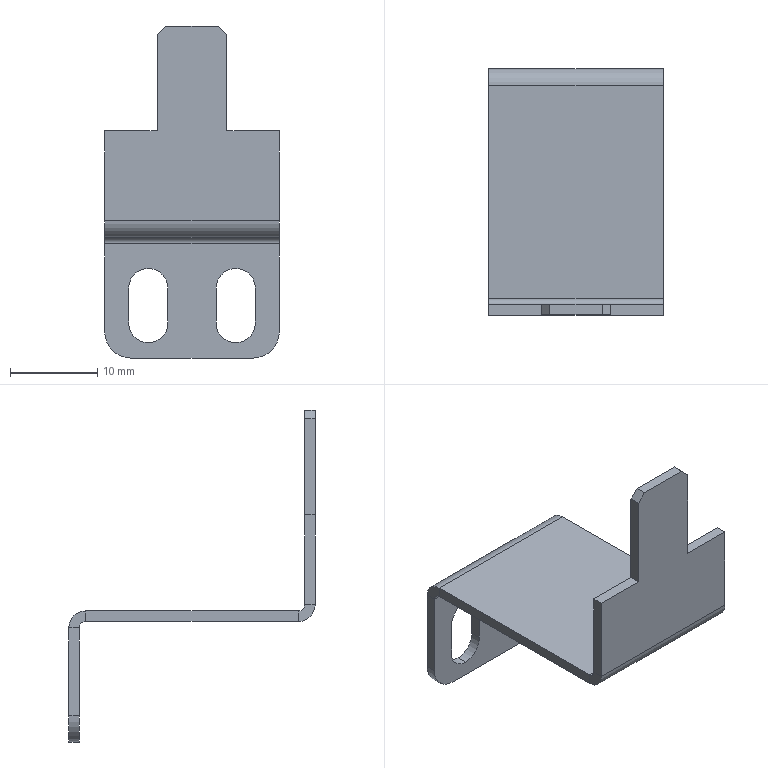Part | SolidWorks | features Chamfer 1, Cut 1, Fillet 1, FlatPattern 1, HoleWzd 1, SMBaseFlange 1, SheetMetal 1 | 1 solid | 40 faces | box 20 x 28.2 x 38 mm | volume 1272 mm3 | plane 28 | cylinder 12 | commonest cylinder face diameters 4.5 x6 1.473 x2 3.873 x2 6 x2
STEP:
#1=CARTESIAN_POINT('',(17.25,27.,-34.));
#2=VERTEX_POINT('',#1);
#3=CARTESIAN_POINT('',(15.,27.,-36.25));
#4=VERTEX_POINT('',#3);
#5=CARTESIAN_POINT('',(15.,27.,-34.));
#6=DIRECTION('',(0.,1.,0.));
#7=DIRECTION('',(0.,0.,1.));
#8=AXIS2_PLACEMENT_3D('',#5,#6,#7);
#9=CIRCLE('',#8,2.25);
#10=EDGE_CURVE('',#2,#4,#9,.T.);
#11=ORIENTED_EDGE('',*,*,#10,.T.);
#12=CARTESIAN_POINT('',(15.,25.8,-36.25));
#13=VERTEX_POINT('',#12);
#14=CARTESIAN_POINT('',(15.,25.8,-36.25));
#15=DIRECTION('',(0.,-1.,0.));
#16=VECTOR('',#15,1000.);
#17=LINE('',#14,#16);
#18=EDGE_CURVE('',#4,#13,#17,.T.);
#19=ORIENTED_EDGE('',*,*,#18,.T.);
#20=CARTESIAN_POINT('',(17.25,25.8,-34.));
#21=VERTEX_POINT('',#20);
#22=CARTESIAN_POINT('',(15.,25.8,-34.));
#23=DIRECTION('',(0.,-1.,0.));
#24=DIRECTION('',(0.,0.,-1.));
#25=AXIS2_PLACEMENT_3D('',#22,#23,#24);
#26=CIRCLE('',#25,2.25);
#27=EDGE_CURVE('',#13,#21,#26,.T.);
#28=ORIENTED_EDGE('',*,*,#27,.T.);
#29=CARTESIAN_POINT('',(17.25,40.8,-34.));
#30=DIRECTION('',(0.,1.,0.));
#31=VECTOR('',#30,1000.);
#32=LINE('',#29,#31);
#33=EDGE_CURVE('',#21,#2,#32,.T.);
#34=ORIENTED_EDGE('',*,*,#33,.T.);
#35=EDGE_LOOP('',(#11,#19,#28,#34));
#36=FACE_OUTER_BOUND('',#35,.T.);
#37=CARTESIAN_POINT('',(15.,25.8,-34.));
#38=DIRECTION('',(0.,-1.,0.));
#39=DIRECTION('',(0.,0.,-1.));
#40=AXIS2_PLACEMENT_3D('',#37,#38,#39);
#41=CYLINDRICAL_SURFACE('',#40,2.25);
#42=ADVANCED_FACE('',(#36),#41,.F.);
#43=CARTESIAN_POINT('',(7.25,27.,-34.));
#44=VERTEX_POINT('',#43);
#45=CARTESIAN_POINT('',(5.,27.,-36.25));
#46=VERTEX_POINT('',#45);
#47=CARTESIAN_POINT('',(5.,27.,-34.));
#48=DIRECTION('',(0.,1.,0.));
#49=DIRECTION('',(0.,0.,1.));
#50=AXIS2_PLACEMENT_3D('',#47,#48,#49);
#51=CIRCLE('',#50,2.25);
#52=EDGE_CURVE('',#44,#46,#51,.T.);
#53=ORIENTED_EDGE('',*,*,#52,.T.);
#54=CARTESIAN_POINT('',(5.,25.8,-36.25));
#55=VERTEX_POINT('',#54);
#56=CARTESIAN_POINT('',(5.,25.8,-36.25));
#57=DIRECTION('',(0.,-1.,0.));
#58=VECTOR('',#57,1000.);
#59=LINE('',#56,#58);
#60=EDGE_CURVE('',#46,#55,#59,.T.);
#61=ORIENTED_EDGE('',*,*,#60,.T.);
#62=CARTESIAN_POINT('',(7.25,25.8,-34.));
#63=VERTEX_POINT('',#62);
#64=CARTESIAN_POINT('',(5.,25.8,-34.));
#65=DIRECTION('',(0.,-1.,0.));
#66=DIRECTION('',(0.,0.,-1.));
#67=AXIS2_PLACEMENT_3D('',#64,#65,#66);
#68=CIRCLE('',#67,2.25);
#69=EDGE_CURVE('',#55,#63,#68,.T.);
#70=ORIENTED_EDGE('',*,*,#69,.T.);
#71=CARTESIAN_POINT('',(7.25,40.8,-34.));
#72=DIRECTION('',(0.,1.,0.));
#73=VECTOR('',#72,1000.);
#74=LINE('',#71,#73);
#75=EDGE_CURVE('',#63,#44,#74,.T.);
#76=ORIENTED_EDGE('',*,*,#75,.T.);
#77=EDGE_LOOP('',(#53,#61,#70,#76));
#78=FACE_OUTER_BOUND('',#77,.T.);
#79=CARTESIAN_POINT('',(5.,25.8,-34.));
#80=DIRECTION('',(0.,-1.,0.));
#81=DIRECTION('',(0.,0.,-1.));
#82=AXIS2_PLACEMENT_3D('',#79,#80,#81);
#83=CYLINDRICAL_SURFACE('',#82,2.25);
#84=ADVANCED_FACE('',(#78),#83,.F.);
#85=ORIENTED_EDGE('',*,*,#10,.F.);
#86=CARTESIAN_POINT('',(17.25,27.,-30.));
#87=VERTEX_POINT('',#86);
#88=CARTESIAN_POINT('',(17.25,27.,-23.));
#89=DIRECTION('',(0.,0.,1.));
#90=VECTOR('',#89,1000.);
#91=LINE('',#88,#90);
#92=EDGE_CURVE('',#2,#87,#91,.T.);
#93=ORIENTED_EDGE('',*,*,#92,.T.);
#94=CARTESIAN_POINT('',(12.75,27.,-30.));
#95=VERTEX_POINT('',#94);
#96=CARTESIAN_POINT('',(15.,27.,-30.));
#97=DIRECTION('',(0.,1.,0.));
#98=DIRECTION('',(0.,0.,1.));
#99=AXIS2_PLACEMENT_3D('',#96,#97,#98);
#100=CIRCLE('',#99,2.25);
#101=EDGE_CURVE('',#95,#87,#100,.T.);
#102=ORIENTED_EDGE('',*,*,#101,.F.);
#103=CARTESIAN_POINT('',(12.75,27.,-34.));
#104=VERTEX_POINT('',#103);
#105=CARTESIAN_POINT('',(12.75,27.,-23.));
#106=DIRECTION('',(0.,0.,1.));
#107=VECTOR('',#106,1000.);
#108=LINE('',#105,#107);
#109=EDGE_CURVE('',#104,#95,#108,.T.);
#110=ORIENTED_EDGE('',*,*,#109,.F.);
#111=CARTESIAN_POINT('',(15.,27.,-34.));
#112=DIRECTION('',(0.,1.,0.));
#113=DIRECTION('',(0.,0.,1.));
#114=AXIS2_PLACEMENT_3D('',#111,#112,#113);
#115=CIRCLE('',#114,2.25);
#116=EDGE_CURVE('',#4,#104,#115,.T.);
#117=ORIENTED_EDGE('',*,*,#116,.F.);
#118=EDGE_LOOP('',(#85,#93,#102,#110,#117));
#119=FACE_BOUND('',#118,.T.);
#120=CARTESIAN_POINT('',(17.,27.,-38.));
#121=VERTEX_POINT('',#120);
#122=CARTESIAN_POINT('',(3.,27.,-38.));
#123=VERTEX_POINT('',#122);
#124=CARTESIAN_POINT('',(20.,27.,-38.));
#125=DIRECTION('',(-1.,0.,0.));
#126=VECTOR('',#125,1000.);
#127=LINE('',#124,#126);
#128=EDGE_CURVE('',#121,#123,#127,.T.);
#129=ORIENTED_EDGE('',*,*,#128,.T.);
#130=CARTESIAN_POINT('',(0.,27.,-35.));
#131=VERTEX_POINT('',#130);
#132=CARTESIAN_POINT('',(3.,27.,-35.));
#133=DIRECTION('',(0.,1.,0.));
#134=DIRECTION('',(0.,0.,1.));
#135=AXIS2_PLACEMENT_3D('',#132,#133,#134);
#136=CIRCLE('',#135,3.);
#137=EDGE_CURVE('',#123,#131,#136,.T.);
#138=ORIENTED_EDGE('',*,*,#137,.T.);
#139=CARTESIAN_POINT('',(0.,27.,-24.937));
#140=VERTEX_POINT('',#139);
#141=CARTESIAN_POINT('',(0.,27.,-23.));
#142=DIRECTION('',(0.,0.,-1.));
#143=VECTOR('',#142,1000.);
#144=LINE('',#141,#143);
#145=EDGE_CURVE('',#140,#131,#144,.T.);
#146=ORIENTED_EDGE('',*,*,#145,.F.);
#147=CARTESIAN_POINT('',(20.,27.,-24.937));
#148=VERTEX_POINT('',#147);
#149=CARTESIAN_POINT('',(20.,27.,-24.937));
#150=DIRECTION('',(-1.,0.,0.));
#151=VECTOR('',#150,1000.);
#152=LINE('',#149,#151);
#153=EDGE_CURVE('',#148,#140,#152,.T.);
#154=ORIENTED_EDGE('',*,*,#153,.F.);
#155=CARTESIAN_POINT('',(20.,27.,-35.));
#156=VERTEX_POINT('',#155);
#157=CARTESIAN_POINT('',(20.,27.,-23.));
#158=DIRECTION('',(0.,0.,-1.));
#159=VECTOR('',#158,1000.);
#160=LINE('',#157,#159);
#161=EDGE_CURVE('',#148,#156,#160,.T.);
#162=ORIENTED_EDGE('',*,*,#161,.T.);
#163=CARTESIAN_POINT('',(17.,27.,-35.));
#164=DIRECTION('',(0.,1.,0.));
#165=DIRECTION('',(0.,0.,1.));
#166=AXIS2_PLACEMENT_3D('',#163,#164,#165);
#167=CIRCLE('',#166,3.);
#168=EDGE_CURVE('',#156,#121,#167,.T.);
#169=ORIENTED_EDGE('',*,*,#168,.T.);
#170=EDGE_LOOP('',(#129,#138,#146,#154,#162,#169));
#171=FACE_OUTER_BOUND('',#170,.T.);
#172=ORIENTED_EDGE('',*,*,#52,.F.);
#173=CARTESIAN_POINT('',(7.25,27.,-30.));
#174=VERTEX_POINT('',#173);
#175=CARTESIAN_POINT('',(7.25,27.,-23.));
#176=DIRECTION('',(0.,0.,1.));
#177=VECTOR('',#176,1000.);
#178=LINE('',#175,#177);
#179=EDGE_CURVE('',#44,#174,#178,.T.);
#180=ORIENTED_EDGE('',*,*,#179,.T.);
#181=CARTESIAN_POINT('',(2.75,27.,-30.));
#182=VERTEX_POINT('',#181);
#183=CARTESIAN_POINT('',(5.,27.,-30.));
#184=DIRECTION('',(0.,1.,0.));
#185=DIRECTION('',(0.,0.,1.));
#186=AXIS2_PLACEMENT_3D('',#183,#184,#185);
#187=CIRCLE('',#186,2.25);
#188=EDGE_CURVE('',#182,#174,#187,.T.);
#189=ORIENTED_EDGE('',*,*,#188,.F.);
#190=CARTESIAN_POINT('',(2.75,27.,-34.));
#191=VERTEX_POINT('',#190);
#192=CARTESIAN_POINT('',(2.75,27.,-23.));
#193=DIRECTION('',(0.,0.,1.));
#194=VECTOR('',#193,1000.);
#195=LINE('',#192,#194);
#196=EDGE_CURVE('',#191,#182,#195,.T.);
#197=ORIENTED_EDGE('',*,*,#196,.F.);
#198=CARTESIAN_POINT('',(5.,27.,-34.));
#199=DIRECTION('',(0.,1.,0.));
#200=DIRECTION('',(0.,0.,1.));
#201=AXIS2_PLACEMENT_3D('',#198,#199,#200);
#202=CIRCLE('',#201,2.25);
#203=EDGE_CURVE('',#46,#191,#202,.T.);
#204=ORIENTED_EDGE('',*,*,#203,.F.);
#205=EDGE_LOOP('',(#172,#180,#189,#197,#204));
#206=FACE_BOUND('',#205,.T.);
#207=CARTESIAN_POINT('',(20.,27.,-23.));
#208=DIRECTION('',(0.,1.,0.));
#209=DIRECTION('',(0.,0.,1.));
#210=AXIS2_PLACEMENT_3D('',#207,#208,#209);
#211=PLANE('',#210);
#212=ADVANCED_FACE('',(#119,#171,#206),#211,.T.);
#213=CARTESIAN_POINT('',(20.,0.7366,-23.));
#214=VERTEX_POINT('',#213);
#215=CARTESIAN_POINT('',(20.,0.7366,-24.2));
#216=VERTEX_POINT('',#215);
#217=CARTESIAN_POINT('',(20.,0.7366,-23.));
#218=DIRECTION('',(0.,0.,-1.));
#219=VECTOR('',#218,1000.);
#220=LINE('',#217,#219);
#221=EDGE_CURVE('',#214,#216,#220,.T.);
#222=ORIENTED_EDGE('',*,*,#221,.F.);
#223=CARTESIAN_POINT('',(20.,0.,-22.263));
#224=VERTEX_POINT('',#223);
#225=CARTESIAN_POINT('',(20.,0.7366,-22.263));
#226=DIRECTION('',(1.,0.,0.));
#227=DIRECTION('',(0.,0.,1.));
#228=AXIS2_PLACEMENT_3D('',#225,#226,#227);
#229=CIRCLE('',#228,0.7366);
#230=EDGE_CURVE('',#224,#214,#229,.T.);
#231=ORIENTED_EDGE('',*,*,#230,.F.);
#232=CARTESIAN_POINT('',(20.,-1.2,-22.263));
#233=VERTEX_POINT('',#232);
#234=CARTESIAN_POINT('',(20.,-1.2,-22.263));
#235=DIRECTION('',(0.,1.,0.));
#236=VECTOR('',#235,1000.);
#237=LINE('',#234,#236);
#238=EDGE_CURVE('',#233,#224,#237,.T.);
#239=ORIENTED_EDGE('',*,*,#238,.F.);
#240=CARTESIAN_POINT('',(20.,0.7366,-22.263));
#241=DIRECTION('',(1.,0.,0.));
#242=DIRECTION('',(0.,0.,-1.));
#243=AXIS2_PLACEMENT_3D('',#240,#241,#242);
#244=CIRCLE('',#243,1.937);
#245=EDGE_CURVE('',#233,#216,#244,.T.);
#246=ORIENTED_EDGE('',*,*,#245,.T.);
#247=EDGE_LOOP('',(#222,#231,#239,#246));
#248=FACE_OUTER_BOUND('',#247,.T.);
#249=CARTESIAN_POINT('',(20.,0.7366,-23.));
#250=DIRECTION('',(1.,0.,0.));
#251=DIRECTION('',(0.,0.,-1.));
#252=AXIS2_PLACEMENT_3D('',#249,#250,#251);
#253=PLANE('',#252);
#254=ADVANCED_FACE('',(#248),#253,.T.);
#255=CARTESIAN_POINT('',(20.,25.063,-23.));
#256=VERTEX_POINT('',#255);
#257=CARTESIAN_POINT('',(20.,0.,-23.));
#258=DIRECTION('',(0.,1.,0.));
#259=VECTOR('',#258,1000.);
#260=LINE('',#257,#259);
#261=EDGE_CURVE('',#214,#256,#260,.T.);
#262=ORIENTED_EDGE('',*,*,#261,.F.);
#263=ORIENTED_EDGE('',*,*,#221,.T.);
#264=CARTESIAN_POINT('',(20.,25.063,-24.2));
#265=VERTEX_POINT('',#264);
#266=CARTESIAN_POINT('',(20.,0.,-24.2));
#267=DIRECTION('',(0.,1.,0.));
#268=VECTOR('',#267,1000.);
#269=LINE('',#266,#268);
#270=EDGE_CURVE('',#216,#265,#269,.T.);
#271=ORIENTED_EDGE('',*,*,#270,.T.);
#272=CARTESIAN_POINT('',(20.,25.063,-24.2));
#273=DIRECTION('',(0.,0.,1.));
#274=VECTOR('',#273,1000.);
#275=LINE('',#272,#274);
#276=EDGE_CURVE('',#265,#256,#275,.T.);
#277=ORIENTED_EDGE('',*,*,#276,.T.);
#278=EDGE_LOOP('',(#262,#263,#271,#277));
#279=FACE_OUTER_BOUND('',#278,.T.);
#280=CARTESIAN_POINT('',(20.,-1.2,-22.263));
#281=DIRECTION('',(1.,0.,0.));
#282=DIRECTION('',(0.,0.,-1.));
#283=AXIS2_PLACEMENT_3D('',#280,#281,#282);
#284=PLANE('',#283);
#285=ADVANCED_FACE('',(#279),#284,.T.);
#286=CARTESIAN_POINT('',(0.,0.,-22.263));
#287=VERTEX_POINT('',#286);
#288=CARTESIAN_POINT('',(0.,-1.2,-22.263));
#289=VERTEX_POINT('',#288);
#290=CARTESIAN_POINT('',(0.,0.,-22.263));
#291=DIRECTION('',(0.,-1.,0.));
#292=VECTOR('',#291,1000.);
#293=LINE('',#290,#292);
#294=EDGE_CURVE('',#287,#289,#293,.T.);
#295=ORIENTED_EDGE('',*,*,#294,.F.);
#296=CARTESIAN_POINT('',(0.,0.7366,-23.));
#297=VERTEX_POINT('',#296);
#298=CARTESIAN_POINT('',(0.,0.7366,-22.263));
#299=DIRECTION('',(1.,0.,0.));
#300=DIRECTION('',(0.,0.,1.));
#301=AXIS2_PLACEMENT_3D('',#298,#299,#300);
#302=CIRCLE('',#301,0.7366);
#303=EDGE_CURVE('',#287,#297,#302,.T.);
#304=ORIENTED_EDGE('',*,*,#303,.T.);
#305=CARTESIAN_POINT('',(0.,0.7366,-24.2));
#306=VERTEX_POINT('',#305);
#307=CARTESIAN_POINT('',(0.,0.7366,-24.2));
#308=DIRECTION('',(0.,0.,1.));
#309=VECTOR('',#308,1000.);
#310=LINE('',#307,#309);
#311=EDGE_CURVE('',#306,#297,#310,.T.);
#312=ORIENTED_EDGE('',*,*,#311,.F.);
#313=CARTESIAN_POINT('',(0.,0.7366,-22.263));
#314=DIRECTION('',(1.,0.,0.));
#315=DIRECTION('',(0.,0.,-1.));
#316=AXIS2_PLACEMENT_3D('',#313,#314,#315);
#317=CIRCLE('',#316,1.937);
#318=EDGE_CURVE('',#289,#306,#317,.T.);
#319=ORIENTED_EDGE('',*,*,#318,.F.);
#320=EDGE_LOOP('',(#295,#304,#312,#319));
#321=FACE_OUTER_BOUND('',#320,.T.);
#322=CARTESIAN_POINT('',(0.,0.,-22.263));
#323=DIRECTION('',(-1.,0.,0.));
#324=DIRECTION('',(0.,0.,1.));
#325=AXIS2_PLACEMENT_3D('',#322,#323,#324);
#326=PLANE('',#325);
#327=ADVANCED_FACE('',(#321),#326,.T.);
#328=CARTESIAN_POINT('',(0.,0.,-12.));
#329=VERTEX_POINT('',#328);
#330=CARTESIAN_POINT('',(0.,-1.2,-12.));
#331=VERTEX_POINT('',#330);
#332=CARTESIAN_POINT('',(0.,27.,-12.));
#333=DIRECTION('',(0.,-1.,0.));
#334=VECTOR('',#333,1000.);
#335=LINE('',#332,#334);
#336=EDGE_CURVE('',#329,#331,#335,.T.);
#337=ORIENTED_EDGE('',*,*,#336,.F.);
#338=CARTESIAN_POINT('',(0.,0.,0.));
#339=DIRECTION('',(0.,0.,-1.));
#340=VECTOR('',#339,1000.);
#341=LINE('',#338,#340);
#342=EDGE_CURVE('',#329,#287,#341,.T.);
#343=ORIENTED_EDGE('',*,*,#342,.T.);
#344=ORIENTED_EDGE('',*,*,#294,.T.);
#345=CARTESIAN_POINT('',(0.,-1.2,0.));
#346=DIRECTION('',(0.,0.,-1.));
#347=VECTOR('',#346,1000.);
#348=LINE('',#345,#347);
#349=EDGE_CURVE('',#331,#289,#348,.T.);
#350=ORIENTED_EDGE('',*,*,#349,.F.);
#351=EDGE_LOOP('',(#337,#343,#344,#350));
#352=FACE_OUTER_BOUND('',#351,.T.);
#353=CARTESIAN_POINT('',(0.,0.7366,-24.2));
#354=DIRECTION('',(-1.,0.,0.));
#355=DIRECTION('',(0.,0.,1.));
#356=AXIS2_PLACEMENT_3D('',#353,#354,#355);
#357=PLANE('',#356);
#358=ADVANCED_FACE('',(#352),#357,.T.);
#359=CARTESIAN_POINT('',(20.,25.8,-24.937));
#360=VERTEX_POINT('',#359);
#361=CARTESIAN_POINT('',(20.,27.,-24.937));
#362=DIRECTION('',(0.,-1.,0.));
#363=VECTOR('',#362,1000.);
#364=LINE('',#361,#363);
#365=EDGE_CURVE('',#148,#360,#364,.T.);
#366=ORIENTED_EDGE('',*,*,#365,.F.);
#367=CARTESIAN_POINT('',(20.,25.063,-24.937));
#368=DIRECTION('',(-1.,0.,0.));
#369=DIRECTION('',(0.,0.,-1.));
#370=AXIS2_PLACEMENT_3D('',#367,#368,#369);
#371=CIRCLE('',#370,1.937);
#372=EDGE_CURVE('',#256,#148,#371,.T.);
#373=ORIENTED_EDGE('',*,*,#372,.F.);
#374=ORIENTED_EDGE('',*,*,#276,.F.);
#375=CARTESIAN_POINT('',(20.,25.063,-24.937));
#376=DIRECTION('',(-1.,0.,0.));
#377=DIRECTION('',(0.,0.,-1.));
#378=AXIS2_PLACEMENT_3D('',#375,#376,#377);
#379=CIRCLE('',#378,0.7366);
#380=EDGE_CURVE('',#265,#360,#379,.T.);
#381=ORIENTED_EDGE('',*,*,#380,.T.);
#382=EDGE_LOOP('',(#366,#373,#374,#381));
#383=FACE_OUTER_BOUND('',#382,.T.);
#384=CARTESIAN_POINT('',(20.,27.,-24.937));
#385=DIRECTION('',(1.,0.,0.));
#386=DIRECTION('',(0.,0.,-1.));
#387=AXIS2_PLACEMENT_3D('',#384,#385,#386);
#388=PLANE('',#387);
#389=ADVANCED_FACE('',(#383),#388,.T.);
#390=CARTESIAN_POINT('',(20.,25.8,-35.));
#391=VERTEX_POINT('',#390);
#392=CARTESIAN_POINT('',(20.,25.8,-23.));
#393=DIRECTION('',(0.,0.,-1.));
#394=VECTOR('',#393,1000.);
#395=LINE('',#392,#394);
#396=EDGE_CURVE('',#360,#391,#395,.T.);
#397=ORIENTED_EDGE('',*,*,#396,.T.);
#398=CARTESIAN_POINT('',(20.,25.063,-35.));
#399=DIRECTION('',(0.,1.,0.));
#400=VECTOR('',#399,1000.);
#401=LINE('',#398,#400);
#402=EDGE_CURVE('',#391,#156,#401,.T.);
#403=ORIENTED_EDGE('',*,*,#402,.T.);
#404=ORIENTED_EDGE('',*,*,#161,.F.);
#405=ORIENTED_EDGE('',*,*,#365,.T.);
#406=EDGE_LOOP('',(#397,#403,#404,#405));
#407=FACE_OUTER_BOUND('',#406,.T.);
#408=CARTESIAN_POINT('',(20.,25.063,-24.2));
#409=DIRECTION('',(1.,0.,0.));
#410=DIRECTION('',(0.,0.,-1.));
#411=AXIS2_PLACEMENT_3D('',#408,#409,#410);
#412=PLANE('',#411);
#413=ADVANCED_FACE('',(#407),#412,.T.);
#414=CARTESIAN_POINT('',(0.,25.063,-23.));
#415=VERTEX_POINT('',#414);
#416=CARTESIAN_POINT('',(0.,25.063,-24.2));
#417=VERTEX_POINT('',#416);
#418=CARTESIAN_POINT('',(0.,25.063,-23.));
#419=DIRECTION('',(0.,0.,-1.));
#420=VECTOR('',#419,1000.);
#421=LINE('',#418,#420);
#422=EDGE_CURVE('',#415,#417,#421,.T.);
#423=ORIENTED_EDGE('',*,*,#422,.F.);
#424=CARTESIAN_POINT('',(0.,25.063,-24.937));
#425=DIRECTION('',(-1.,0.,0.));
#426=DIRECTION('',(0.,0.,-1.));
#427=AXIS2_PLACEMENT_3D('',#424,#425,#426);
#428=CIRCLE('',#427,1.937);
#429=EDGE_CURVE('',#415,#140,#428,.T.);
#430=ORIENTED_EDGE('',*,*,#429,.T.);
#431=CARTESIAN_POINT('',(0.,25.8,-24.937));
#432=VERTEX_POINT('',#431);
#433=CARTESIAN_POINT('',(0.,25.8,-24.937));
#434=DIRECTION('',(0.,1.,0.));
#435=VECTOR('',#434,1000.);
#436=LINE('',#433,#435);
#437=EDGE_CURVE('',#432,#140,#436,.T.);
#438=ORIENTED_EDGE('',*,*,#437,.F.);
#439=CARTESIAN_POINT('',(0.,25.063,-24.937));
#440=DIRECTION('',(-1.,0.,0.));
#441=DIRECTION('',(0.,0.,-1.));
#442=AXIS2_PLACEMENT_3D('',#439,#440,#441);
#443=CIRCLE('',#442,0.7366);
#444=EDGE_CURVE('',#417,#432,#443,.T.);
#445=ORIENTED_EDGE('',*,*,#444,.F.);
#446=EDGE_LOOP('',(#423,#430,#438,#445));
#447=FACE_OUTER_BOUND('',#446,.T.);
#448=CARTESIAN_POINT('',(0.,25.063,-23.));
#449=DIRECTION('',(-1.,0.,0.));
#450=DIRECTION('',(0.,0.,1.));
#451=AXIS2_PLACEMENT_3D('',#448,#449,#450);
#452=PLANE('',#451);
#453=ADVANCED_FACE('',(#447),#452,.T.);
#454=CARTESIAN_POINT('',(0.,0.,-23.));
#455=DIRECTION('',(0.,1.,0.));
#456=VECTOR('',#455,1000.);
#457=LINE('',#454,#456);
#458=EDGE_CURVE('',#297,#415,#457,.T.);
#459=ORIENTED_EDGE('',*,*,#458,.T.);
#460=ORIENTED_EDGE('',*,*,#422,.T.);
#461=CARTESIAN_POINT('',(0.,0.,-24.2));
#462=DIRECTION('',(0.,1.,0.));
#463=VECTOR('',#462,1000.);
#464=LINE('',#461,#463);
#465=EDGE_CURVE('',#306,#417,#464,.T.);
#466=ORIENTED_EDGE('',*,*,#465,.F.);
#467=ORIENTED_EDGE('',*,*,#311,.T.);
#468=EDGE_LOOP('',(#459,#460,#466,#467));
#469=FACE_OUTER_BOUND('',#468,.T.);
#470=CARTESIAN_POINT('',(0.,25.8,-24.937));
#471=DIRECTION('',(-1.,0.,0.));
#472=DIRECTION('',(0.,0.,1.));
#473=AXIS2_PLACEMENT_3D('',#470,#471,#472);
#474=PLANE('',#473);
#475=ADVANCED_FACE('',(#469),#474,.T.);
#476=CARTESIAN_POINT('',(17.25,25.8,-30.));
#477=VERTEX_POINT('',#476);
#478=CARTESIAN_POINT('',(17.25,25.8,-30.));
#479=DIRECTION('',(0.,0.,-1.));
#480=VECTOR('',#479,1000.);
#481=LINE('',#478,#480);
#482=EDGE_CURVE('',#477,#21,#481,.T.);
#483=ORIENTED_EDGE('',*,*,#482,.T.);
#484=ORIENTED_EDGE('',*,*,#27,.F.);
#485=CARTESIAN_POINT('',(12.75,25.8,-34.));
#486=VERTEX_POINT('',#485);
#487=CARTESIAN_POINT('',(15.,25.8,-34.));
#488=DIRECTION('',(0.,-1.,0.));
#489=DIRECTION('',(0.,0.,-1.));
#490=AXIS2_PLACEMENT_3D('',#487,#488,#489);
#491=CIRCLE('',#490,2.25);
#492=EDGE_CURVE('',#486,#13,#491,.T.);
#493=ORIENTED_EDGE('',*,*,#492,.F.);
#494=CARTESIAN_POINT('',(12.75,25.8,-30.));
#495=VERTEX_POINT('',#494);
#496=CARTESIAN_POINT('',(12.75,25.8,-30.));
#497=DIRECTION('',(0.,0.,-1.));
#498=VECTOR('',#497,1000.);
#499=LINE('',#496,#498);
#500=EDGE_CURVE('',#495,#486,#499,.T.);
#501=ORIENTED_EDGE('',*,*,#500,.F.);
#502=CARTESIAN_POINT('',(15.,25.8,-30.));
#503=DIRECTION('',(0.,-1.,0.));
#504=DIRECTION('',(0.,0.,-1.));
#505=AXIS2_PLACEMENT_3D('',#502,#503,#504);
#506=CIRCLE('',#505,2.25);
#507=EDGE_CURVE('',#477,#495,#506,.T.);
#508=ORIENTED_EDGE('',*,*,#507,.F.);
#509=EDGE_LOOP('',(#483,#484,#493,#501,#508));
#510=FACE_BOUND('',#509,.T.);
#511=CARTESIAN_POINT('',(2.75,25.8,-30.));
#512=VERTEX_POINT('',#511);
#513=CARTESIAN_POINT('',(2.75,25.8,-34.));
#514=VERTEX_POINT('',#513);
#515=CARTESIAN_POINT('',(2.75,25.8,-30.));
#516=DIRECTION('',(0.,0.,-1.));
#517=VECTOR('',#516,1000.);
#518=LINE('',#515,#517);
#519=EDGE_CURVE('',#512,#514,#518,.T.);
#520=ORIENTED_EDGE('',*,*,#519,.F.);
#521=CARTESIAN_POINT('',(7.25,25.8,-30.));
#522=VERTEX_POINT('',#521);
#523=CARTESIAN_POINT('',(5.,25.8,-30.));
#524=DIRECTION('',(0.,-1.,0.));
#525=DIRECTION('',(0.,0.,-1.));
#526=AXIS2_PLACEMENT_3D('',#523,#524,#525);
#527=CIRCLE('',#526,2.25);
#528=EDGE_CURVE('',#522,#512,#527,.T.);
#529=ORIENTED_EDGE('',*,*,#528,.F.);
#530=CARTESIAN_POINT('',(7.25,25.8,-30.));
#531=DIRECTION('',(0.,0.,-1.));
#532=VECTOR('',#531,1000.);
#533=LINE('',#530,#532);
#534=EDGE_CURVE('',#522,#63,#533,.T.);
#535=ORIENTED_EDGE('',*,*,#534,.T.);
#536=ORIENTED_EDGE('',*,*,#69,.F.);
#537=CARTESIAN_POINT('',(5.,25.8,-34.));
#538=DIRECTION('',(0.,-1.,0.));
#539=DIRECTION('',(0.,0.,-1.));
#540=AXIS2_PLACEMENT_3D('',#537,#538,#539);
#541=CIRCLE('',#540,2.25);
#542=EDGE_CURVE('',#514,#55,#541,.T.);
#543=ORIENTED_EDGE('',*,*,#542,.F.);
#544=EDGE_LOOP('',(#520,#529,#535,#536,#543));
#545=FACE_BOUND('',#544,.T.);
#546=CARTESIAN_POINT('',(0.,25.8,-35.));
#547=VERTEX_POINT('',#546);
#548=CARTESIAN_POINT('',(0.,25.8,-23.));
#549=DIRECTION('',(0.,0.,-1.));
#550=VECTOR('',#549,1000.);
#551=LINE('',#548,#550);
#552=EDGE_CURVE('',#432,#547,#551,.T.);
#553=ORIENTED_EDGE('',*,*,#552,.T.);
#554=CARTESIAN_POINT('',(3.,25.8,-38.));
#555=VERTEX_POINT('',#554);
#556=CARTESIAN_POINT('',(3.,25.8,-35.));
#557=DIRECTION('',(0.,-1.,0.));
#558=DIRECTION('',(0.,0.,1.));
#559=AXIS2_PLACEMENT_3D('',#556,#557,#558);
#560=CIRCLE('',#559,3.);
#561=EDGE_CURVE('',#547,#555,#560,.T.);
#562=ORIENTED_EDGE('',*,*,#561,.T.);
#563=CARTESIAN_POINT('',(17.,25.8,-38.));
#564=VERTEX_POINT('',#563);
#565=CARTESIAN_POINT('',(20.,25.8,-38.));
#566=DIRECTION('',(-1.,0.,0.));
#567=VECTOR('',#566,1000.);
#568=LINE('',#565,#567);
#569=EDGE_CURVE('',#564,#555,#568,.T.);
#570=ORIENTED_EDGE('',*,*,#569,.F.);
#571=CARTESIAN_POINT('',(17.,25.8,-35.));
#572=DIRECTION('',(0.,-1.,0.));
#573=DIRECTION('',(0.,0.,1.));
#574=AXIS2_PLACEMENT_3D('',#571,#572,#573);
#575=CIRCLE('',#574,3.);
#576=EDGE_CURVE('',#564,#391,#575,.T.);
#577=ORIENTED_EDGE('',*,*,#576,.T.);
#578=ORIENTED_EDGE('',*,*,#396,.F.);
#579=CARTESIAN_POINT('',(20.,25.8,-24.937));
#580=DIRECTION('',(-1.,0.,0.));
#581=VECTOR('',#580,1000.);
#582=LINE('',#579,#581);
#583=EDGE_CURVE('',#360,#432,#582,.T.);
#584=ORIENTED_EDGE('',*,*,#583,.T.);
#585=EDGE_LOOP('',(#553,#562,#570,#577,#578,#584));
#586=FACE_OUTER_BOUND('',#585,.T.);
#587=CARTESIAN_POINT('',(20.,25.8,-23.));
#588=DIRECTION('',(0.,1.,0.));
#589=DIRECTION('',(0.,0.,1.));
#590=AXIS2_PLACEMENT_3D('',#587,#588,#589);
#591=PLANE('',#590);
#592=ADVANCED_FACE('',(#510,#545,#586),#591,.F.);
#593=ORIENTED_EDGE('',*,*,#569,.T.);
#594=CARTESIAN_POINT('',(3.,27.,-38.));
#595=DIRECTION('',(0.,1.,0.));
#596=VECTOR('',#595,1000.);
#597=LINE('',#594,#596);
#598=EDGE_CURVE('',#555,#123,#597,.T.);
#599=ORIENTED_EDGE('',*,*,#598,.T.);
#600=ORIENTED_EDGE('',*,*,#128,.F.);
#601=CARTESIAN_POINT('',(17.,27.,-38.));
#602=DIRECTION('',(0.,-1.,0.));
#603=VECTOR('',#602,1000.);
#604=LINE('',#601,#603);
#605=EDGE_CURVE('',#121,#564,#604,.T.);
#606=ORIENTED_EDGE('',*,*,#605,.T.);
#607=EDGE_LOOP('',(#593,#599,#600,#606));
#608=FACE_OUTER_BOUND('',#607,.T.);
#609=CARTESIAN_POINT('',(20.,27.,-38.));
#610=DIRECTION('',(0.,0.,-1.));
#611=DIRECTION('',(-1.,0.,0.));
#612=AXIS2_PLACEMENT_3D('',#609,#610,#611);
#613=PLANE('',#612);
#614=ADVANCED_FACE('',(#608),#613,.T.);
#615=ORIENTED_EDGE('',*,*,#429,.F.);
#616=CARTESIAN_POINT('',(20.,25.063,-23.));
#617=DIRECTION('',(-1.,0.,0.));
#618=VECTOR('',#617,1000.);
#619=LINE('',#616,#618);
#620=EDGE_CURVE('',#256,#415,#619,.T.);
#621=ORIENTED_EDGE('',*,*,#620,.F.);
#622=ORIENTED_EDGE('',*,*,#372,.T.);
#623=ORIENTED_EDGE('',*,*,#153,.T.);
#624=EDGE_LOOP('',(#615,#621,#622,#623));
#625=FACE_OUTER_BOUND('',#624,.T.);
#626=CARTESIAN_POINT('',(20.,25.063,-24.937));
#627=DIRECTION('',(-1.,0.,0.));
#628=DIRECTION('',(0.,0.,1.));
#629=AXIS2_PLACEMENT_3D('',#626,#627,#628);
#630=CYLINDRICAL_SURFACE('',#629,1.937);
#631=ADVANCED_FACE('',(#625),#630,.T.);
#632=ORIENTED_EDGE('',*,*,#458,.F.);
#633=CARTESIAN_POINT('',(20.,0.7366,-23.));
#634=DIRECTION('',(-1.,0.,0.));
#635=VECTOR('',#634,1000.);
#636=LINE('',#633,#635);
#637=EDGE_CURVE('',#214,#297,#636,.T.);
#638=ORIENTED_EDGE('',*,*,#637,.F.);
#639=ORIENTED_EDGE('',*,*,#261,.T.);
#640=ORIENTED_EDGE('',*,*,#620,.T.);
#641=EDGE_LOOP('',(#632,#638,#639,#640));
#642=FACE_OUTER_BOUND('',#641,.T.);
#643=CARTESIAN_POINT('',(20.,0.,-23.));
#644=DIRECTION('',(0.,0.,1.));
#645=DIRECTION('',(1.,0.,0.));
#646=AXIS2_PLACEMENT_3D('',#643,#644,#645);
#647=PLANE('',#646);
#648=ADVANCED_FACE('',(#642),#647,.T.);
#649=ORIENTED_EDGE('',*,*,#303,.F.);
#650=CARTESIAN_POINT('',(20.,0.,-22.263));
#651=DIRECTION('',(-1.,0.,0.));
#652=VECTOR('',#651,1000.);
#653=LINE('',#650,#652);
#654=EDGE_CURVE('',#224,#287,#653,.T.);
#655=ORIENTED_EDGE('',*,*,#654,.F.);
#656=ORIENTED_EDGE('',*,*,#230,.T.);
#657=ORIENTED_EDGE('',*,*,#637,.T.);
#658=EDGE_LOOP('',(#649,#655,#656,#657));
#659=FACE_OUTER_BOUND('',#658,.T.);
#660=CARTESIAN_POINT('',(20.,0.7366,-22.263));
#661=DIRECTION('',(-1.,0.,0.));
#662=DIRECTION('',(0.,0.,1.));
#663=AXIS2_PLACEMENT_3D('',#660,#661,#662);
#664=CYLINDRICAL_SURFACE('',#663,0.7366);
#665=ADVANCED_FACE('',(#659),#664,.F.);
#666=CARTESIAN_POINT('',(6.,0.,-1.));
#667=VERTEX_POINT('',#666);
#668=CARTESIAN_POINT('',(6.,0.,-12.));
#669=VERTEX_POINT('',#668);
#670=CARTESIAN_POINT('',(6.,0.,0.));
#671=DIRECTION('',(0.,0.,-1.));
#672=VECTOR('',#671,1000.);
#673=LINE('',#670,#672);
#674=EDGE_CURVE('',#667,#669,#673,.T.);
#675=ORIENTED_EDGE('',*,*,#674,.F.);
#676=CARTESIAN_POINT('',(7.,0.,0.));
#677=VERTEX_POINT('',#676);
#678=CARTESIAN_POINT('',(13.5,0.,6.5));
#679=DIRECTION('',(0.7071,0.,0.7071));
#680=VECTOR('',#679,1000.);
#681=LINE('',#678,#680);
#682=EDGE_CURVE('',#667,#677,#681,.T.);
#683=ORIENTED_EDGE('',*,*,#682,.T.);
#684=CARTESIAN_POINT('',(13.,0.,0.));
#685=VERTEX_POINT('',#684);
#686=CARTESIAN_POINT('',(20.,0.,0.));
#687=DIRECTION('',(-1.,0.,0.));
#688=VECTOR('',#687,1000.);
#689=LINE('',#686,#688);
#690=EDGE_CURVE('',#685,#677,#689,.T.);
#691=ORIENTED_EDGE('',*,*,#690,.F.);
#692=CARTESIAN_POINT('',(14.,0.,-1.));
#693=VERTEX_POINT('',#692);
#694=CARTESIAN_POINT('',(16.5,0.,-3.5));
#695=DIRECTION('',(0.7071,0.,-0.7071));
#696=VECTOR('',#695,1000.);
#697=LINE('',#694,#696);
#698=EDGE_CURVE('',#685,#693,#697,.T.);
#699=ORIENTED_EDGE('',*,*,#698,.T.);
#700=CARTESIAN_POINT('',(14.,0.,-12.));
#701=VERTEX_POINT('',#700);
#702=CARTESIAN_POINT('',(14.,0.,0.));
#703=DIRECTION('',(0.,0.,1.));
#704=VECTOR('',#703,1000.);
#705=LINE('',#702,#704);
#706=EDGE_CURVE('',#701,#693,#705,.T.);
#707=ORIENTED_EDGE('',*,*,#706,.F.);
#708=CARTESIAN_POINT('',(20.,0.,-12.));
#709=VERTEX_POINT('',#708);
#710=CARTESIAN_POINT('',(20.,0.,-12.));
#711=DIRECTION('',(-1.,0.,0.));
#712=VECTOR('',#711,1000.);
#713=LINE('',#710,#712);
#714=EDGE_CURVE('',#709,#701,#713,.T.);
#715=ORIENTED_EDGE('',*,*,#714,.F.);
#716=CARTESIAN_POINT('',(20.,0.,0.));
#717=DIRECTION('',(0.,0.,-1.));
#718=VECTOR('',#717,1000.);
#719=LINE('',#716,#718);
#720=EDGE_CURVE('',#709,#224,#719,.T.);
#721=ORIENTED_EDGE('',*,*,#720,.T.);
#722=ORIENTED_EDGE('',*,*,#654,.T.);
#723=ORIENTED_EDGE('',*,*,#342,.F.);
#724=CARTESIAN_POINT('',(20.,0.,-12.));
#725=DIRECTION('',(-1.,0.,0.));
#726=VECTOR('',#725,1000.);
#727=LINE('',#724,#726);
#728=EDGE_CURVE('',#669,#329,#727,.T.);
#729=ORIENTED_EDGE('',*,*,#728,.F.);
#730=EDGE_LOOP('',(#675,#683,#691,#699,#707,#715,#721,#722,#723,#729));
#731=FACE_OUTER_BOUND('',#730,.T.);
#732=CARTESIAN_POINT('',(20.,0.,0.));
#733=DIRECTION('',(0.,1.,0.));
#734=DIRECTION('',(0.,0.,1.));
#735=AXIS2_PLACEMENT_3D('',#732,#733,#734);
#736=PLANE('',#735);
#737=ADVANCED_FACE('',(#731),#736,.T.);
#738=ORIENTED_EDGE('',*,*,#690,.T.);
#739=CARTESIAN_POINT('',(7.,-1.2,0.));
#740=VERTEX_POINT('',#739);
#741=CARTESIAN_POINT('',(7.,-1.2,0.));
#742=DIRECTION('',(0.,-1.,0.));
#743=VECTOR('',#742,1000.);
#744=LINE('',#741,#743);
#745=EDGE_CURVE('',#677,#740,#744,.T.);
#746=ORIENTED_EDGE('',*,*,#745,.T.);
#747=CARTESIAN_POINT('',(13.,-1.2,0.));
#748=VERTEX_POINT('',#747);
#749=CARTESIAN_POINT('',(20.,-1.2,0.));
#750=DIRECTION('',(-1.,0.,0.));
#751=VECTOR('',#750,1000.);
#752=LINE('',#749,#751);
#753=EDGE_CURVE('',#748,#740,#752,.T.);
#754=ORIENTED_EDGE('',*,*,#753,.F.);
#755=CARTESIAN_POINT('',(13.,0.,0.));
#756=DIRECTION('',(0.,1.,0.));
#757=VECTOR('',#756,1000.);
#758=LINE('',#755,#757);
#759=EDGE_CURVE('',#748,#685,#758,.T.);
#760=ORIENTED_EDGE('',*,*,#759,.T.);
#761=EDGE_LOOP('',(#738,#746,#754,#760));
#762=FACE_OUTER_BOUND('',#761,.T.);
#763=CARTESIAN_POINT('',(20.,-1.2,0.));
#764=DIRECTION('',(0.,0.,1.));
#765=DIRECTION('',(1.,0.,0.));
#766=AXIS2_PLACEMENT_3D('',#763,#764,#765);
#767=PLANE('',#766);
#768=ADVANCED_FACE('',(#762),#767,.T.);
#769=ORIENTED_EDGE('',*,*,#753,.T.);
#770=CARTESIAN_POINT('',(6.,-1.2,-1.));
#771=VERTEX_POINT('',#770);
#772=CARTESIAN_POINT('',(7.,-1.2,0.));
#773=DIRECTION('',(-0.7071,0.,-0.7071));
#774=VECTOR('',#773,1000.);
#775=LINE('',#772,#774);
#776=EDGE_CURVE('',#740,#771,#775,.T.);
#777=ORIENTED_EDGE('',*,*,#776,.T.);
#778=CARTESIAN_POINT('',(6.,-1.2,-12.));
#779=VERTEX_POINT('',#778);
#780=CARTESIAN_POINT('',(6.,-1.2,0.));
#781=DIRECTION('',(0.,0.,1.));
#782=VECTOR('',#781,1000.);
#783=LINE('',#780,#782);
#784=EDGE_CURVE('',#779,#771,#783,.T.);
#785=ORIENTED_EDGE('',*,*,#784,.F.);
#786=CARTESIAN_POINT('',(0.,-1.2,-12.));
#787=DIRECTION('',(1.,0.,0.));
#788=VECTOR('',#787,1000.);
#789=LINE('',#786,#788);
#790=EDGE_CURVE('',#331,#779,#789,.T.);
#791=ORIENTED_EDGE('',*,*,#790,.F.);
#792=ORIENTED_EDGE('',*,*,#349,.T.);
#793=CARTESIAN_POINT('',(20.,-1.2,-22.263));
#794=DIRECTION('',(-1.,0.,0.));
#795=VECTOR('',#794,1000.);
#796=LINE('',#793,#795);
#797=EDGE_CURVE('',#233,#289,#796,.T.);
#798=ORIENTED_EDGE('',*,*,#797,.F.);
#799=CARTESIAN_POINT('',(20.,-1.2,-12.));
#800=VERTEX_POINT('',#799);
#801=CARTESIAN_POINT('',(20.,-1.2,0.));
#802=DIRECTION('',(0.,0.,-1.));
#803=VECTOR('',#802,1000.);
#804=LINE('',#801,#803);
#805=EDGE_CURVE('',#800,#233,#804,.T.);
#806=ORIENTED_EDGE('',*,*,#805,.F.);
#807=CARTESIAN_POINT('',(14.,-1.2,-12.));
#808=VERTEX_POINT('',#807);
#809=CARTESIAN_POINT('',(20.,-1.2,-12.));
#810=DIRECTION('',(1.,0.,0.));
#811=VECTOR('',#810,1000.);
#812=LINE('',#809,#811);
#813=EDGE_CURVE('',#808,#800,#812,.T.);
#814=ORIENTED_EDGE('',*,*,#813,.F.);
#815=CARTESIAN_POINT('',(14.,-1.2,-1.));
#816=VERTEX_POINT('',#815);
#817=CARTESIAN_POINT('',(14.,-1.2,0.));
#818=DIRECTION('',(0.,0.,-1.));
#819=VECTOR('',#818,1000.);
#820=LINE('',#817,#819);
#821=EDGE_CURVE('',#816,#808,#820,.T.);
#822=ORIENTED_EDGE('',*,*,#821,.F.);
#823=CARTESIAN_POINT('',(14.,-1.2,-1.));
#824=DIRECTION('',(-0.7071,0.,0.7071));
#825=VECTOR('',#824,1000.);
#826=LINE('',#823,#825);
#827=EDGE_CURVE('',#816,#748,#826,.T.);
#828=ORIENTED_EDGE('',*,*,#827,.T.);
#829=EDGE_LOOP('',(#769,#777,#785,#791,#792,#798,#806,#814,#822,#828));
#830=FACE_OUTER_BOUND('',#829,.T.);
#831=CARTESIAN_POINT('',(20.,-1.2,0.));
#832=DIRECTION('',(0.,1.,0.));
#833=DIRECTION('',(0.,0.,1.));
#834=AXIS2_PLACEMENT_3D('',#831,#832,#833);
#835=PLANE('',#834);
#836=ADVANCED_FACE('',(#830),#835,.F.);
#837=ORIENTED_EDGE('',*,*,#318,.T.);
#838=CARTESIAN_POINT('',(20.,0.7366,-24.2));
#839=DIRECTION('',(-1.,0.,0.));
#840=VECTOR('',#839,1000.);
#841=LINE('',#838,#840);
#842=EDGE_CURVE('',#216,#306,#841,.T.);
#843=ORIENTED_EDGE('',*,*,#842,.F.);
#844=ORIENTED_EDGE('',*,*,#245,.F.);
#845=ORIENTED_EDGE('',*,*,#797,.T.);
#846=EDGE_LOOP('',(#837,#843,#844,#845));
#847=FACE_OUTER_BOUND('',#846,.T.);
#848=CARTESIAN_POINT('',(20.,0.7366,-22.263));
#849=DIRECTION('',(-1.,0.,0.));
#850=DIRECTION('',(0.,0.,1.));
#851=AXIS2_PLACEMENT_3D('',#848,#849,#850);
#852=CYLINDRICAL_SURFACE('',#851,1.937);
#853=ADVANCED_FACE('',(#847),#852,.T.);
#854=ORIENTED_EDGE('',*,*,#465,.T.);
#855=CARTESIAN_POINT('',(20.,25.063,-24.2));
#856=DIRECTION('',(-1.,0.,0.));
#857=VECTOR('',#856,1000.);
#858=LINE('',#855,#857);
#859=EDGE_CURVE('',#265,#417,#858,.T.);
#860=ORIENTED_EDGE('',*,*,#859,.F.);
#861=ORIENTED_EDGE('',*,*,#270,.F.);
#862=ORIENTED_EDGE('',*,*,#842,.T.);
#863=EDGE_LOOP('',(#854,#860,#861,#862));
#864=FACE_OUTER_BOUND('',#863,.T.);
#865=CARTESIAN_POINT('',(20.,0.,-24.2));
#866=DIRECTION('',(0.,0.,1.));
#867=DIRECTION('',(1.,0.,0.));
#868=AXIS2_PLACEMENT_3D('',#865,#866,#867);
#869=PLANE('',#868);
#870=ADVANCED_FACE('',(#864),#869,.F.);
#871=ORIENTED_EDGE('',*,*,#444,.T.);
#872=ORIENTED_EDGE('',*,*,#583,.F.);
#873=ORIENTED_EDGE('',*,*,#380,.F.);
#874=ORIENTED_EDGE('',*,*,#859,.T.);
#875=EDGE_LOOP('',(#871,#872,#873,#874));
#876=FACE_OUTER_BOUND('',#875,.T.);
#877=CARTESIAN_POINT('',(20.,25.063,-24.937));
#878=DIRECTION('',(-1.,0.,0.));
#879=DIRECTION('',(0.,0.,1.));
#880=AXIS2_PLACEMENT_3D('',#877,#878,#879);
#881=CYLINDRICAL_SURFACE('',#880,0.7366);
#882=ADVANCED_FACE('',(#876),#881,.F.);
#883=CARTESIAN_POINT('',(20.,25.063,-12.));
#884=DIRECTION('',(0.,1.,0.));
#885=VECTOR('',#884,1000.);
#886=LINE('',#883,#885);
#887=EDGE_CURVE('',#800,#709,#886,.T.);
#888=ORIENTED_EDGE('',*,*,#887,.F.);
#889=ORIENTED_EDGE('',*,*,#805,.T.);
#890=ORIENTED_EDGE('',*,*,#238,.T.);
#891=ORIENTED_EDGE('',*,*,#720,.F.);
#892=EDGE_LOOP('',(#888,#889,#890,#891));
#893=FACE_OUTER_BOUND('',#892,.T.);
#894=CARTESIAN_POINT('',(20.,25.063,-24.937));
#895=DIRECTION('',(1.,0.,0.));
#896=DIRECTION('',(0.,0.,-1.));
#897=AXIS2_PLACEMENT_3D('',#894,#895,#896);
#898=PLANE('',#897);
#899=ADVANCED_FACE('',(#893),#898,.T.);
#900=ORIENTED_EDGE('',*,*,#145,.T.);
#901=CARTESIAN_POINT('',(0.,25.8,-35.));
#902=DIRECTION('',(0.,-1.,0.));
#903=VECTOR('',#902,1000.);
#904=LINE('',#901,#903);
#905=EDGE_CURVE('',#131,#547,#904,.T.);
#906=ORIENTED_EDGE('',*,*,#905,.T.);
#907=ORIENTED_EDGE('',*,*,#552,.F.);
#908=ORIENTED_EDGE('',*,*,#437,.T.);
#909=EDGE_LOOP('',(#900,#906,#907,#908));
#910=FACE_OUTER_BOUND('',#909,.T.);
#911=CARTESIAN_POINT('',(0.,25.063,-24.937));
#912=DIRECTION('',(1.,0.,0.));
#913=DIRECTION('',(0.,0.,-1.));
#914=AXIS2_PLACEMENT_3D('',#911,#912,#913);
#915=PLANE('',#914);
#916=ADVANCED_FACE('',(#910),#915,.F.);
#917=ORIENTED_EDGE('',*,*,#714,.T.);
#918=CARTESIAN_POINT('',(14.,27.,-12.));
#919=DIRECTION('',(0.,-1.,0.));
#920=VECTOR('',#919,1000.);
#921=LINE('',#918,#920);
#922=EDGE_CURVE('',#701,#808,#921,.T.);
#923=ORIENTED_EDGE('',*,*,#922,.T.);
#924=ORIENTED_EDGE('',*,*,#813,.T.);
#925=ORIENTED_EDGE('',*,*,#887,.T.);
#926=EDGE_LOOP('',(#917,#923,#924,#925));
#927=FACE_OUTER_BOUND('',#926,.T.);
#928=CARTESIAN_POINT('',(20.,27.,-12.));
#929=DIRECTION('',(0.,0.,-1.));
#930=DIRECTION('',(-1.,0.,0.));
#931=AXIS2_PLACEMENT_3D('',#928,#929,#930);
#932=PLANE('',#931);
#933=ADVANCED_FACE('',(#927),#932,.F.);
#934=ORIENTED_EDGE('',*,*,#706,.T.);
#935=CARTESIAN_POINT('',(14.,-1.2,-1.));
#936=DIRECTION('',(0.,-1.,0.));
#937=VECTOR('',#936,1000.);
#938=LINE('',#935,#937);
#939=EDGE_CURVE('',#693,#816,#938,.T.);
#940=ORIENTED_EDGE('',*,*,#939,.T.);
#941=ORIENTED_EDGE('',*,*,#821,.T.);
#942=ORIENTED_EDGE('',*,*,#922,.F.);
#943=EDGE_LOOP('',(#934,#940,#941,#942));
#944=FACE_OUTER_BOUND('',#943,.T.);
#945=CARTESIAN_POINT('',(14.,27.,0.));
#946=DIRECTION('',(-1.,0.,0.));
#947=DIRECTION('',(0.,0.,1.));
#948=AXIS2_PLACEMENT_3D('',#945,#946,#947);
#949=PLANE('',#948);
#950=ADVANCED_FACE('',(#944),#949,.F.);
#951=ORIENTED_EDGE('',*,*,#784,.T.);
#952=CARTESIAN_POINT('',(6.,0.,-1.));
#953=DIRECTION('',(0.,1.,0.));
#954=VECTOR('',#953,1000.);
#955=LINE('',#952,#954);
#956=EDGE_CURVE('',#771,#667,#955,.T.);
#957=ORIENTED_EDGE('',*,*,#956,.T.);
#958=ORIENTED_EDGE('',*,*,#674,.T.);
#959=CARTESIAN_POINT('',(6.,27.,-12.));
#960=DIRECTION('',(0.,-1.,0.));
#961=VECTOR('',#960,1000.);
#962=LINE('',#959,#961);
#963=EDGE_CURVE('',#669,#779,#962,.T.);
#964=ORIENTED_EDGE('',*,*,#963,.T.);
#965=EDGE_LOOP('',(#951,#957,#958,#964));
#966=FACE_OUTER_BOUND('',#965,.T.);
#967=CARTESIAN_POINT('',(6.,27.,0.));
#968=DIRECTION('',(1.,0.,0.));
#969=DIRECTION('',(0.,0.,-1.));
#970=AXIS2_PLACEMENT_3D('',#967,#968,#969);
#971=PLANE('',#970);
#972=ADVANCED_FACE('',(#966),#971,.F.);
#973=ORIENTED_EDGE('',*,*,#728,.T.);
#974=ORIENTED_EDGE('',*,*,#336,.T.);
#975=ORIENTED_EDGE('',*,*,#790,.T.);
#976=ORIENTED_EDGE('',*,*,#963,.F.);
#977=EDGE_LOOP('',(#973,#974,#975,#976));
#978=FACE_OUTER_BOUND('',#977,.T.);
#979=CARTESIAN_POINT('',(0.,27.,-12.));
#980=DIRECTION('',(0.,0.,-1.));
#981=DIRECTION('',(-1.,0.,0.));
#982=AXIS2_PLACEMENT_3D('',#979,#980,#981);
#983=PLANE('',#982);
#984=ADVANCED_FACE('',(#978),#983,.F.);
#985=ORIENTED_EDGE('',*,*,#60,.F.);
#986=ORIENTED_EDGE('',*,*,#203,.T.);
#987=CARTESIAN_POINT('',(2.75,25.8,-34.));
#988=DIRECTION('',(0.,1.,0.));
#989=VECTOR('',#988,1000.);
#990=LINE('',#987,#989);
#991=EDGE_CURVE('',#514,#191,#990,.T.);
#992=ORIENTED_EDGE('',*,*,#991,.F.);
#993=ORIENTED_EDGE('',*,*,#542,.T.);
#994=EDGE_LOOP('',(#985,#986,#992,#993));
#995=FACE_OUTER_BOUND('',#994,.T.);
#996=CARTESIAN_POINT('',(5.,25.8,-34.));
#997=DIRECTION('',(0.,-1.,0.));
#998=DIRECTION('',(0.,0.,-1.));
#999=AXIS2_PLACEMENT_3D('',#996,#997,#998);
#1000=CYLINDRICAL_SURFACE('',#999,2.25);
#1001=ADVANCED_FACE('',(#995),#1000,.F.);
#1002=ORIENTED_EDGE('',*,*,#188,.T.);
#1003=CARTESIAN_POINT('',(7.25,40.8,-30.));
#1004=DIRECTION('',(0.,1.,0.));
#1005=VECTOR('',#1004,1000.);
#1006=LINE('',#1003,#1005);
#1007=EDGE_CURVE('',#522,#174,#1006,.T.);
#1008=ORIENTED_EDGE('',*,*,#1007,.F.);
#1009=ORIENTED_EDGE('',*,*,#528,.T.);
#1010=CARTESIAN_POINT('',(2.75,25.8,-30.));
#1011=DIRECTION('',(0.,-1.,0.));
#1012=VECTOR('',#1011,1000.);
#1013=LINE('',#1010,#1012);
#1014=EDGE_CURVE('',#182,#512,#1013,.T.);
#1015=ORIENTED_EDGE('',*,*,#1014,.F.);
#1016=EDGE_LOOP('',(#1002,#1008,#1009,#1015));
#1017=FACE_OUTER_BOUND('',#1016,.T.);
#1018=CARTESIAN_POINT('',(5.,25.8,-30.));
#1019=DIRECTION('',(0.,-1.,0.));
#1020=DIRECTION('',(0.,0.,-1.));
#1021=AXIS2_PLACEMENT_3D('',#1018,#1019,#1020);
#1022=CYLINDRICAL_SURFACE('',#1021,2.25);
#1023=ADVANCED_FACE('',(#1017),#1022,.F.);
#1024=ORIENTED_EDGE('',*,*,#75,.F.);
#1025=ORIENTED_EDGE('',*,*,#534,.F.);
#1026=ORIENTED_EDGE('',*,*,#1007,.T.);
#1027=ORIENTED_EDGE('',*,*,#179,.F.);
#1028=EDGE_LOOP('',(#1024,#1025,#1026,#1027));
#1029=FACE_OUTER_BOUND('',#1028,.T.);
#1030=CARTESIAN_POINT('',(7.25,40.8,-30.));
#1031=DIRECTION('',(-1.,0.,0.));
#1032=DIRECTION('',(0.,-1.,0.));
#1033=AXIS2_PLACEMENT_3D('',#1030,#1031,#1032);
#1034=PLANE('',#1033);
#1035=ADVANCED_FACE('',(#1029),#1034,.T.);
#1036=ORIENTED_EDGE('',*,*,#196,.T.);
#1037=ORIENTED_EDGE('',*,*,#1014,.T.);
#1038=ORIENTED_EDGE('',*,*,#519,.T.);
#1039=ORIENTED_EDGE('',*,*,#991,.T.);
#1040=EDGE_LOOP('',(#1036,#1037,#1038,#1039));
#1041=FACE_OUTER_BOUND('',#1040,.T.);
#1042=CARTESIAN_POINT('',(2.75,25.8,-30.));
#1043=DIRECTION('',(-1.,0.,0.));
#1044=DIRECTION('',(0.,0.,1.));
#1045=AXIS2_PLACEMENT_3D('',#1042,#1043,#1044);
#1046=PLANE('',#1045);
#1047=ADVANCED_FACE('',(#1041),#1046,.F.);
#1048=ORIENTED_EDGE('',*,*,#18,.F.);
#1049=ORIENTED_EDGE('',*,*,#116,.T.);
#1050=CARTESIAN_POINT('',(12.75,25.8,-34.));
#1051=DIRECTION('',(0.,1.,0.));
#1052=VECTOR('',#1051,1000.);
#1053=LINE('',#1050,#1052);
#1054=EDGE_CURVE('',#486,#104,#1053,.T.);
#1055=ORIENTED_EDGE('',*,*,#1054,.F.);
#1056=ORIENTED_EDGE('',*,*,#492,.T.);
#1057=EDGE_LOOP('',(#1048,#1049,#1055,#1056));
#1058=FACE_OUTER_BOUND('',#1057,.T.);
#1059=CARTESIAN_POINT('',(15.,25.8,-34.));
#1060=DIRECTION('',(0.,-1.,0.));
#1061=DIRECTION('',(0.,0.,-1.));
#1062=AXIS2_PLACEMENT_3D('',#1059,#1060,#1061);
#1063=CYLINDRICAL_SURFACE('',#1062,2.25);
#1064=ADVANCED_FACE('',(#1058),#1063,.F.);
#1065=ORIENTED_EDGE('',*,*,#101,.T.);
#1066=CARTESIAN_POINT('',(17.25,40.8,-30.));
#1067=DIRECTION('',(0.,1.,0.));
#1068=VECTOR('',#1067,1000.);
#1069=LINE('',#1066,#1068);
#1070=EDGE_CURVE('',#477,#87,#1069,.T.);
#1071=ORIENTED_EDGE('',*,*,#1070,.F.);
#1072=ORIENTED_EDGE('',*,*,#507,.T.);
#1073=CARTESIAN_POINT('',(12.75,25.8,-30.));
#1074=DIRECTION('',(0.,-1.,0.));
#1075=VECTOR('',#1074,1000.);
#1076=LINE('',#1073,#1075);
#1077=EDGE_CURVE('',#95,#495,#1076,.T.);
#1078=ORIENTED_EDGE('',*,*,#1077,.F.);
#1079=EDGE_LOOP('',(#1065,#1071,#1072,#1078));
#1080=FACE_OUTER_BOUND('',#1079,.T.);
#1081=CARTESIAN_POINT('',(15.,25.8,-30.));
#1082=DIRECTION('',(0.,-1.,0.));
#1083=DIRECTION('',(0.,0.,-1.));
#1084=AXIS2_PLACEMENT_3D('',#1081,#1082,#1083);
#1085=CYLINDRICAL_SURFACE('',#1084,2.25);
#1086=ADVANCED_FACE('',(#1080),#1085,.F.);
#1087=ORIENTED_EDGE('',*,*,#33,.F.);
#1088=ORIENTED_EDGE('',*,*,#482,.F.);
#1089=ORIENTED_EDGE('',*,*,#1070,.T.);
#1090=ORIENTED_EDGE('',*,*,#92,.F.);
#1091=EDGE_LOOP('',(#1087,#1088,#1089,#1090));
#1092=FACE_OUTER_BOUND('',#1091,.T.);
#1093=CARTESIAN_POINT('',(17.25,40.8,-30.));
#1094=DIRECTION('',(-1.,0.,0.));
#1095=DIRECTION('',(0.,-1.,0.));
#1096=AXIS2_PLACEMENT_3D('',#1093,#1094,#1095);
#1097=PLANE('',#1096);
#1098=ADVANCED_FACE('',(#1092),#1097,.T.);
#1099=ORIENTED_EDGE('',*,*,#109,.T.);
#1100=ORIENTED_EDGE('',*,*,#1077,.T.);
#1101=ORIENTED_EDGE('',*,*,#500,.T.);
#1102=ORIENTED_EDGE('',*,*,#1054,.T.);
#1103=EDGE_LOOP('',(#1099,#1100,#1101,#1102));
#1104=FACE_OUTER_BOUND('',#1103,.T.);
#1105=CARTESIAN_POINT('',(12.75,25.8,-30.));
#1106=DIRECTION('',(-1.,0.,0.));
#1107=DIRECTION('',(0.,0.,1.));
#1108=AXIS2_PLACEMENT_3D('',#1105,#1106,#1107);
#1109=PLANE('',#1108);
#1110=ADVANCED_FACE('',(#1104),#1109,.F.);
#1111=ORIENTED_EDGE('',*,*,#137,.F.);
#1112=ORIENTED_EDGE('',*,*,#598,.F.);
#1113=ORIENTED_EDGE('',*,*,#561,.F.);
#1114=ORIENTED_EDGE('',*,*,#905,.F.);
#1115=EDGE_LOOP('',(#1111,#1112,#1113,#1114));
#1116=FACE_OUTER_BOUND('',#1115,.T.);
#1117=CARTESIAN_POINT('',(3.,25.063,-35.));
#1118=DIRECTION('',(0.,1.,0.));
#1119=DIRECTION('',(0.,0.,1.));
#1120=AXIS2_PLACEMENT_3D('',#1117,#1118,#1119);
#1121=CYLINDRICAL_SURFACE('',#1120,3.);
#1122=ADVANCED_FACE('',(#1116),#1121,.T.);
#1123=ORIENTED_EDGE('',*,*,#168,.F.);
#1124=ORIENTED_EDGE('',*,*,#402,.F.);
#1125=ORIENTED_EDGE('',*,*,#576,.F.);
#1126=ORIENTED_EDGE('',*,*,#605,.F.);
#1127=EDGE_LOOP('',(#1123,#1124,#1125,#1126));
#1128=FACE_OUTER_BOUND('',#1127,.T.);
#1129=CARTESIAN_POINT('',(17.,27.,-35.));
#1130=DIRECTION('',(0.,-1.,0.));
#1131=DIRECTION('',(0.,0.,-1.));
#1132=AXIS2_PLACEMENT_3D('',#1129,#1130,#1131);
#1133=CYLINDRICAL_SURFACE('',#1132,3.);
#1134=ADVANCED_FACE('',(#1128),#1133,.T.);
#1135=ORIENTED_EDGE('',*,*,#682,.F.);
#1136=ORIENTED_EDGE('',*,*,#956,.F.);
#1137=ORIENTED_EDGE('',*,*,#776,.F.);
#1138=ORIENTED_EDGE('',*,*,#745,.F.);
#1139=EDGE_LOOP('',(#1135,#1136,#1137,#1138));
#1140=FACE_OUTER_BOUND('',#1139,.T.);
#1141=CARTESIAN_POINT('',(7.,-1.2,0.));
#1142=DIRECTION('',(-0.7071,0.,0.7071));
#1143=DIRECTION('',(0.,1.,0.));
#1144=AXIS2_PLACEMENT_3D('',#1141,#1142,#1143);
#1145=PLANE('',#1144);
#1146=ADVANCED_FACE('',(#1140),#1145,.T.);
#1147=ORIENTED_EDGE('',*,*,#698,.F.);
#1148=ORIENTED_EDGE('',*,*,#759,.F.);
#1149=ORIENTED_EDGE('',*,*,#827,.F.);
#1150=ORIENTED_EDGE('',*,*,#939,.F.);
#1151=EDGE_LOOP('',(#1147,#1148,#1149,#1150));
#1152=FACE_OUTER_BOUND('',#1151,.T.);
#1153=CARTESIAN_POINT('',(14.,27.,-1.));
#1154=DIRECTION('',(0.7071,0.,0.7071));
#1155=DIRECTION('',(0.,1.,0.));
#1156=AXIS2_PLACEMENT_3D('',#1153,#1154,#1155);
#1157=PLANE('',#1156);
#1158=ADVANCED_FACE('',(#1152),#1157,.T.);
#1159=CLOSED_SHELL('',(#42,#84,#212,#254,#285,#327,#358,#389,#413,#453,#475,#592,#614,#631,#648,#665,#737,#768,#836,#853,#870,#882,#899,#916,#933,#950,#972,#984,#1001,#1023,#1035,#1047,#1064,#1086,#1098,#1110,#1122,#1134,#1146,#1158));
#1160=MANIFOLD_SOLID_BREP('',#1159);
#1161=CARTESIAN_POINT('',(0.,0.,0.));
#1162=DIRECTION('',(0.,0.,1.));
#1163=DIRECTION('',(1.,0.,0.));
#1164=AXIS2_PLACEMENT_3D('',#1161,#1162,#1163);
#1165=(LENGTH_UNIT()NAMED_UNIT(*)SI_UNIT(.MILLI.,.METRE.));
#1166=UNCERTAINTY_MEASURE_WITH_UNIT(LENGTH_MEASURE(0.00001),#1165,'','');
#1167=(NAMED_UNIT(*)PLANE_ANGLE_UNIT()SI_UNIT($,.RADIAN.));
#1168=(NAMED_UNIT(*)SI_UNIT($,.STERADIAN.)SOLID_ANGLE_UNIT());
#1169=(GEOMETRIC_REPRESENTATION_CONTEXT(3)GLOBAL_UNCERTAINTY_ASSIGNED_CONTEXT((#1166))GLOBAL_UNIT_ASSIGNED_CONTEXT((#1165,#1167,#1168))REPRESENTATION_CONTEXT('',''));
#1170=ADVANCED_BREP_SHAPE_REPRESENTATION('',(#1160,#1164),#1169);